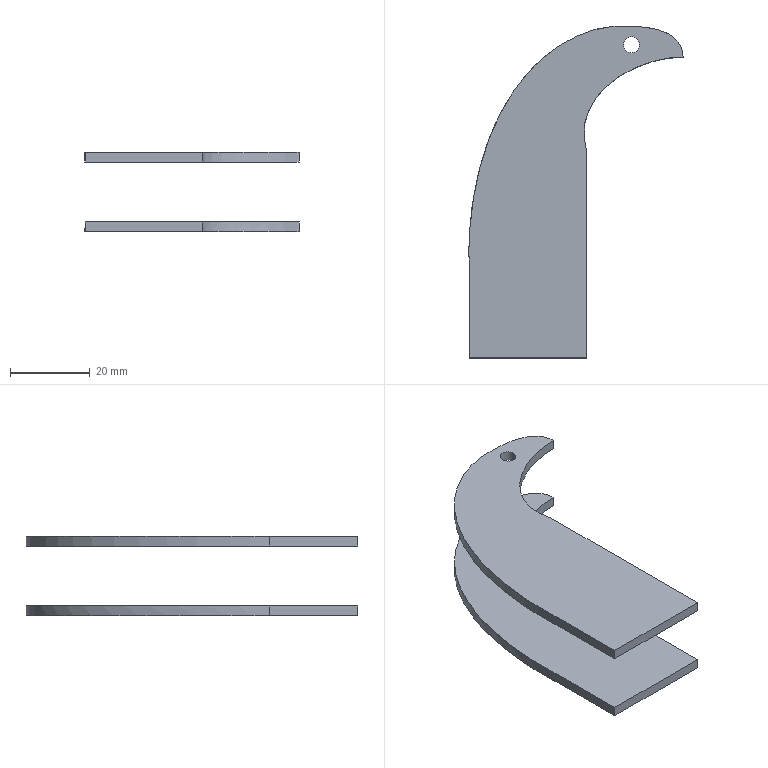Part | SolidWorks | features ICE 2, Extrusion 1 | 2 solids | 18 faces | box 53.74 x 83.25 x 20 mm | volume 11198 mm3 | plane 10 | cylinder 4 | spline 4 | commonest cylinder face diameters 4 x4
STEP:
#1=CARTESIAN_POINT('',(20.268,78.539,-10.));
#2=VERTEX_POINT('',#1);
#3=CARTESIAN_POINT('',(24.268,78.539,-10.));
#4=VERTEX_POINT('',#3);
#5=CARTESIAN_POINT('',(22.268,78.539,-10.));
#6=DIRECTION('',(0.,0.,1.));
#7=DIRECTION('',(1.,0.,0.));
#8=AXIS2_PLACEMENT_3D('',#5,#6,#7);
#9=CIRCLE('',#8,2.);
#10=EDGE_CURVE('',#2,#4,#9,.T.);
#11=ORIENTED_EDGE('',*,*,#10,.F.);
#12=CARTESIAN_POINT('',(20.268,78.539,-7.5));
#13=VERTEX_POINT('',#12);
#14=CARTESIAN_POINT('',(20.268,78.539,-90.));
#15=DIRECTION('',(0.,0.,1.));
#16=VECTOR('',#15,1000.);
#17=LINE('',#14,#16);
#18=EDGE_CURVE('',#2,#13,#17,.T.);
#19=ORIENTED_EDGE('',*,*,#18,.T.);
#20=CARTESIAN_POINT('',(24.268,78.539,-7.5));
#21=VERTEX_POINT('',#20);
#22=CARTESIAN_POINT('',(22.268,78.539,-7.5));
#23=DIRECTION('',(0.,0.,-1.));
#24=DIRECTION('',(-1.,0.,0.));
#25=AXIS2_PLACEMENT_3D('',#22,#23,#24);
#26=CIRCLE('',#25,2.);
#27=EDGE_CURVE('',#21,#13,#26,.T.);
#28=ORIENTED_EDGE('',*,*,#27,.F.);
#29=CARTESIAN_POINT('',(24.268,78.539,-90.));
#30=DIRECTION('',(0.,0.,1.));
#31=VECTOR('',#30,1000.);
#32=LINE('',#29,#31);
#33=EDGE_CURVE('',#4,#21,#32,.T.);
#34=ORIENTED_EDGE('',*,*,#33,.F.);
#35=EDGE_LOOP('',(#11,#19,#28,#34));
#36=FACE_OUTER_BOUND('',#35,.T.);
#37=CARTESIAN_POINT('',(22.268,78.539,-90.));
#38=DIRECTION('',(0.,0.,1.));
#39=DIRECTION('',(1.,0.,0.));
#40=AXIS2_PLACEMENT_3D('',#37,#38,#39);
#41=CYLINDRICAL_SURFACE('',#40,2.);
#42=ADVANCED_FACE('',(#36),#41,.F.);
#43=CARTESIAN_POINT('',(-18.438,0.,-7.5));
#44=VERTEX_POINT('',#43);
#45=CARTESIAN_POINT('',(-18.438,0.,-10.));
#46=VERTEX_POINT('',#45);
#47=CARTESIAN_POINT('',(-18.438,0.,10.));
#48=DIRECTION('',(0.,0.,-1.));
#49=VECTOR('',#48,1000.);
#50=LINE('',#47,#49);
#51=EDGE_CURVE('',#44,#46,#50,.T.);
#52=ORIENTED_EDGE('',*,*,#51,.F.);
#53=CARTESIAN_POINT('',(-18.438,22.25,-7.5));
#54=VERTEX_POINT('',#53);
#55=CARTESIAN_POINT('',(-18.438,0.,-7.5));
#56=DIRECTION('',(0.,1.,0.));
#57=VECTOR('',#56,1000.);
#58=LINE('',#55,#57);
#59=EDGE_CURVE('',#44,#54,#58,.T.);
#60=ORIENTED_EDGE('',*,*,#59,.T.);
#61=CARTESIAN_POINT('',(-18.438,22.25,-10.));
#62=VERTEX_POINT('',#61);
#63=CARTESIAN_POINT('',(-18.438,22.25,10.));
#64=DIRECTION('',(0.,0.,-1.));
#65=VECTOR('',#64,1000.);
#66=LINE('',#63,#65);
#67=EDGE_CURVE('',#54,#62,#66,.T.);
#68=ORIENTED_EDGE('',*,*,#67,.T.);
#69=CARTESIAN_POINT('',(-18.438,0.,-10.));
#70=DIRECTION('',(0.,-1.,0.));
#71=VECTOR('',#70,1000.);
#72=LINE('',#69,#71);
#73=EDGE_CURVE('',#62,#46,#72,.T.);
#74=ORIENTED_EDGE('',*,*,#73,.T.);
#75=EDGE_LOOP('',(#52,#60,#68,#74));
#76=FACE_OUTER_BOUND('',#75,.T.);
#77=CARTESIAN_POINT('',(-18.438,0.,10.));
#78=DIRECTION('',(1.,0.,0.));
#79=DIRECTION('',(0.,0.,-1.));
#80=AXIS2_PLACEMENT_3D('',#77,#78,#79);
#81=PLANE('',#80);
#82=ADVANCED_FACE('',(#76),#81,.F.);
#83=CARTESIAN_POINT('',(10.984,0.,-7.5));
#84=VERTEX_POINT('',#83);
#85=CARTESIAN_POINT('',(10.984,0.,-10.));
#86=VERTEX_POINT('',#85);
#87=CARTESIAN_POINT('',(10.984,0.,10.));
#88=DIRECTION('',(0.,0.,-1.));
#89=VECTOR('',#88,1000.);
#90=LINE('',#87,#89);
#91=EDGE_CURVE('',#84,#86,#90,.T.);
#92=ORIENTED_EDGE('',*,*,#91,.F.);
#93=CARTESIAN_POINT('',(-18.438,0.,-7.5));
#94=DIRECTION('',(-1.,0.,0.));
#95=VECTOR('',#94,1000.);
#96=LINE('',#93,#95);
#97=EDGE_CURVE('',#84,#44,#96,.T.);
#98=ORIENTED_EDGE('',*,*,#97,.T.);
#99=ORIENTED_EDGE('',*,*,#51,.T.);
#100=CARTESIAN_POINT('',(-18.438,0.,-10.));
#101=DIRECTION('',(1.,0.,0.));
#102=VECTOR('',#101,1000.);
#103=LINE('',#100,#102);
#104=EDGE_CURVE('',#46,#86,#103,.T.);
#105=ORIENTED_EDGE('',*,*,#104,.T.);
#106=EDGE_LOOP('',(#92,#98,#99,#105));
#107=FACE_OUTER_BOUND('',#106,.T.);
#108=CARTESIAN_POINT('',(-18.438,0.,10.));
#109=DIRECTION('',(0.,1.,0.));
#110=DIRECTION('',(0.,0.,1.));
#111=AXIS2_PLACEMENT_3D('',#108,#109,#110);
#112=PLANE('',#111);
#113=ADVANCED_FACE('',(#107),#112,.F.);
#114=CARTESIAN_POINT('',(10.984,52.083,-7.5));
#115=VERTEX_POINT('',#114);
#116=CARTESIAN_POINT('',(10.984,52.083,-10.));
#117=VERTEX_POINT('',#116);
#118=CARTESIAN_POINT('',(10.984,52.083,10.));
#119=DIRECTION('',(0.,0.,-1.));
#120=VECTOR('',#119,1000.);
#121=LINE('',#118,#120);
#122=EDGE_CURVE('',#115,#117,#121,.T.);
#123=ORIENTED_EDGE('',*,*,#122,.F.);
#124=CARTESIAN_POINT('',(10.984,52.083,-7.5));
#125=DIRECTION('',(0.,-1.,0.));
#126=VECTOR('',#125,1000.);
#127=LINE('',#124,#126);
#128=EDGE_CURVE('',#115,#84,#127,.T.);
#129=ORIENTED_EDGE('',*,*,#128,.T.);
#130=ORIENTED_EDGE('',*,*,#91,.T.);
#131=CARTESIAN_POINT('',(10.984,52.083,-10.));
#132=DIRECTION('',(0.,1.,0.));
#133=VECTOR('',#132,1000.);
#134=LINE('',#131,#133);
#135=EDGE_CURVE('',#86,#117,#134,.T.);
#136=ORIENTED_EDGE('',*,*,#135,.T.);
#137=EDGE_LOOP('',(#123,#129,#130,#136));
#138=FACE_OUTER_BOUND('',#137,.T.);
#139=CARTESIAN_POINT('',(10.984,52.083,10.));
#140=DIRECTION('',(-1.,0.,0.));
#141=DIRECTION('',(0.,-1.,0.));
#142=AXIS2_PLACEMENT_3D('',#139,#140,#141);
#143=PLANE('',#142);
#144=ADVANCED_FACE('',(#138),#143,.F.);
#145=CARTESIAN_POINT('',(35.215,75.441,-7.5));
#146=VERTEX_POINT('',#145);
#147=CARTESIAN_POINT('',(35.215,75.441,-10.));
#148=VERTEX_POINT('',#147);
#149=CARTESIAN_POINT('',(35.215,75.441,10.));
#150=DIRECTION('',(0.,0.,-1.));
#151=VECTOR('',#150,1000.);
#152=LINE('',#149,#151);
#153=EDGE_CURVE('',#146,#148,#152,.T.);
#154=ORIENTED_EDGE('',*,*,#153,.F.);
#155=CARTESIAN_POINT('',(35.215,75.441,-7.5));
#156=CARTESIAN_POINT('',(23.557,75.598,-7.5));
#157=CARTESIAN_POINT('',(6.934,66.328,-7.5));
#158=CARTESIAN_POINT('',(10.984,52.083,-7.5));
#159=B_SPLINE_CURVE_WITH_KNOTS('',3,(#155,#156,#157,#158),.UNSPECIFIED.,.F.,.F.,(4,4),(0.,1.),.UNSPECIFIED.);
#160=EDGE_CURVE('',#146,#115,#159,.T.);
#161=ORIENTED_EDGE('',*,*,#160,.T.);
#162=ORIENTED_EDGE('',*,*,#122,.T.);
#163=CARTESIAN_POINT('',(10.984,52.083,-10.));
#164=CARTESIAN_POINT('',(6.934,66.328,-10.));
#165=CARTESIAN_POINT('',(23.557,75.598,-10.));
#166=CARTESIAN_POINT('',(35.215,75.441,-10.));
#167=B_SPLINE_CURVE_WITH_KNOTS('',3,(#163,#164,#165,#166),.UNSPECIFIED.,.F.,.F.,(4,4),(0.,1.),.UNSPECIFIED.);
#168=EDGE_CURVE('',#117,#148,#167,.T.);
#169=ORIENTED_EDGE('',*,*,#168,.T.);
#170=EDGE_LOOP('',(#154,#161,#162,#169));
#171=FACE_OUTER_BOUND('',#170,.T.);
#172=CARTESIAN_POINT('',(10.984,52.083,-7.5));
#173=CARTESIAN_POINT('',(10.984,52.083,-10.));
#174=CARTESIAN_POINT('',(6.934,66.328,-7.5));
#175=CARTESIAN_POINT('',(6.934,66.328,-10.));
#176=CARTESIAN_POINT('',(23.557,75.598,-7.5));
#177=CARTESIAN_POINT('',(23.557,75.598,-10.));
#178=CARTESIAN_POINT('',(35.215,75.441,-7.5));
#179=CARTESIAN_POINT('',(35.215,75.441,-10.));
#180=B_SPLINE_SURFACE_WITH_KNOTS('',3,1,((#172,#173),(#174,#175),(#176,#177),(#178,#179)),.UNSPECIFIED.,.F.,.F.,.F.,(4,4),(2,2),(0.,1.),(0.,1.),.UNSPECIFIED.);
#181=ADVANCED_FACE('',(#171),#180,.F.);
#182=ORIENTED_EDGE('',*,*,#67,.F.);
#183=CARTESIAN_POINT('',(-18.438,22.25,-7.5));
#184=CARTESIAN_POINT('',(-19.279,40.919,-7.5));
#185=CARTESIAN_POINT('',(-12.619,70.796,-7.5));
#186=CARTESIAN_POINT('',(13.495,83.4,-7.5));
#187=CARTESIAN_POINT('',(23.092,83.31,-7.5));
#188=CARTESIAN_POINT('',(30.862,82.311,-7.5));
#189=CARTESIAN_POINT('',(35.305,78.999,-7.5));
#190=CARTESIAN_POINT('',(35.215,75.441,-7.5));
#191=B_SPLINE_CURVE_WITH_KNOTS('',3,(#183,#184,#185,#186,#187,#188,#189,#190),.UNSPECIFIED.,.F.,.F.,(4,1,1,1,1,4),(0.,0.6141,0.7591,0.8514,0.9042,1.),.UNSPECIFIED.);
#192=EDGE_CURVE('',#54,#146,#191,.T.);
#193=ORIENTED_EDGE('',*,*,#192,.T.);
#194=ORIENTED_EDGE('',*,*,#153,.T.);
#195=CARTESIAN_POINT('',(35.215,75.441,-10.));
#196=CARTESIAN_POINT('',(35.305,78.999,-10.));
#197=CARTESIAN_POINT('',(30.862,82.311,-10.));
#198=CARTESIAN_POINT('',(23.092,83.31,-10.));
#199=CARTESIAN_POINT('',(13.495,83.4,-10.));
#200=CARTESIAN_POINT('',(-12.619,70.796,-10.));
#201=CARTESIAN_POINT('',(-19.279,40.919,-10.));
#202=CARTESIAN_POINT('',(-18.438,22.25,-10.));
#203=B_SPLINE_CURVE_WITH_KNOTS('',3,(#195,#196,#197,#198,#199,#200,#201,#202),.UNSPECIFIED.,.F.,.F.,(4,1,1,1,1,4),(0.,0.09577,0.1486,0.2409,0.3859,1.),.UNSPECIFIED.);
#204=EDGE_CURVE('',#148,#62,#203,.T.);
#205=ORIENTED_EDGE('',*,*,#204,.T.);
#206=EDGE_LOOP('',(#182,#193,#194,#205));
#207=FACE_OUTER_BOUND('',#206,.T.);
#208=CARTESIAN_POINT('',(35.215,75.441,-7.5));
#209=CARTESIAN_POINT('',(35.215,75.441,-10.));
#210=CARTESIAN_POINT('',(35.305,78.999,-7.5));
#211=CARTESIAN_POINT('',(35.305,78.999,-10.));
#212=CARTESIAN_POINT('',(30.862,82.311,-7.5));
#213=CARTESIAN_POINT('',(30.862,82.311,-10.));
#214=CARTESIAN_POINT('',(23.092,83.31,-7.5));
#215=CARTESIAN_POINT('',(23.092,83.31,-10.));
#216=CARTESIAN_POINT('',(13.495,83.4,-7.5));
#217=CARTESIAN_POINT('',(13.495,83.4,-10.));
#218=CARTESIAN_POINT('',(-12.619,70.796,-7.5));
#219=CARTESIAN_POINT('',(-12.619,70.796,-10.));
#220=CARTESIAN_POINT('',(-19.279,40.919,-7.5));
#221=CARTESIAN_POINT('',(-19.279,40.919,-10.));
#222=CARTESIAN_POINT('',(-18.438,22.25,-7.5));
#223=CARTESIAN_POINT('',(-18.438,22.25,-10.));
#224=B_SPLINE_SURFACE_WITH_KNOTS('',3,1,((#208,#209),(#210,#211),(#212,#213),(#214,#215),(#216,#217),(#218,#219),(#220,#221),(#222,#223)),.UNSPECIFIED.,.F.,.F.,.F.,(4,1,1,1,1,4),(2,2),(0.,0.09577,0.1486,0.2409,0.3859,1.),(0.,1.),.UNSPECIFIED.);
#225=ADVANCED_FACE('',(#207),#224,.F.);
#226=CARTESIAN_POINT('',(22.268,78.539,-10.));
#227=DIRECTION('',(0.,0.,1.));
#228=DIRECTION('',(1.,0.,0.));
#229=AXIS2_PLACEMENT_3D('',#226,#227,#228);
#230=CIRCLE('',#229,2.);
#231=EDGE_CURVE('',#4,#2,#230,.T.);
#232=ORIENTED_EDGE('',*,*,#231,.T.);
#233=ORIENTED_EDGE('',*,*,#10,.T.);
#234=EDGE_LOOP('',(#232,#233));
#235=FACE_BOUND('',#234,.T.);
#236=ORIENTED_EDGE('',*,*,#73,.F.);
#237=ORIENTED_EDGE('',*,*,#204,.F.);
#238=ORIENTED_EDGE('',*,*,#168,.F.);
#239=ORIENTED_EDGE('',*,*,#135,.F.);
#240=ORIENTED_EDGE('',*,*,#104,.F.);
#241=EDGE_LOOP('',(#236,#237,#238,#239,#240));
#242=FACE_OUTER_BOUND('',#241,.T.);
#243=CARTESIAN_POINT('',(-5.594,69.238,-10.));
#244=DIRECTION('',(0.,0.,1.));
#245=DIRECTION('',(1.,0.,0.));
#246=AXIS2_PLACEMENT_3D('',#243,#244,#245);
#247=PLANE('',#246);
#248=ADVANCED_FACE('',(#235,#242),#247,.F.);
#249=ORIENTED_EDGE('',*,*,#27,.T.);
#250=CARTESIAN_POINT('',(22.268,78.539,-7.5));
#251=DIRECTION('',(0.,0.,-1.));
#252=DIRECTION('',(-1.,0.,0.));
#253=AXIS2_PLACEMENT_3D('',#250,#251,#252);
#254=CIRCLE('',#253,2.);
#255=EDGE_CURVE('',#13,#21,#254,.T.);
#256=ORIENTED_EDGE('',*,*,#255,.T.);
#257=EDGE_LOOP('',(#249,#256));
#258=FACE_BOUND('',#257,.T.);
#259=ORIENTED_EDGE('',*,*,#97,.F.);
#260=ORIENTED_EDGE('',*,*,#128,.F.);
#261=ORIENTED_EDGE('',*,*,#160,.F.);
#262=ORIENTED_EDGE('',*,*,#192,.F.);
#263=ORIENTED_EDGE('',*,*,#59,.F.);
#264=EDGE_LOOP('',(#259,#260,#261,#262,#263));
#265=FACE_OUTER_BOUND('',#264,.T.);
#266=CARTESIAN_POINT('',(-50.,-93.589,-7.5));
#267=DIRECTION('',(0.,0.,-1.));
#268=DIRECTION('',(-1.,0.,0.));
#269=AXIS2_PLACEMENT_3D('',#266,#267,#268);
#270=PLANE('',#269);
#271=ADVANCED_FACE('',(#258,#265),#270,.F.);
#272=ORIENTED_EDGE('',*,*,#18,.F.);
#273=ORIENTED_EDGE('',*,*,#231,.F.);
#274=ORIENTED_EDGE('',*,*,#33,.T.);
#275=ORIENTED_EDGE('',*,*,#255,.F.);
#276=EDGE_LOOP('',(#272,#273,#274,#275));
#277=FACE_OUTER_BOUND('',#276,.T.);
#278=CARTESIAN_POINT('',(22.268,78.539,-90.));
#279=DIRECTION('',(0.,0.,1.));
#280=DIRECTION('',(1.,0.,0.));
#281=AXIS2_PLACEMENT_3D('',#278,#279,#280);
#282=CYLINDRICAL_SURFACE('',#281,2.);
#283=ADVANCED_FACE('',(#277),#282,.F.);
#284=CLOSED_SHELL('',(#42,#82,#113,#144,#181,#225,#248,#271,#283));
#285=MANIFOLD_SOLID_BREP('',#284);
#286=CARTESIAN_POINT('',(20.268,78.539,7.5));
#287=VERTEX_POINT('',#286);
#288=CARTESIAN_POINT('',(24.268,78.539,7.5));
#289=VERTEX_POINT('',#288);
#290=CARTESIAN_POINT('',(22.268,78.539,7.5));
#291=DIRECTION('',(0.,0.,1.));
#292=DIRECTION('',(1.,0.,0.));
#293=AXIS2_PLACEMENT_3D('',#290,#291,#292);
#294=CIRCLE('',#293,2.);
#295=EDGE_CURVE('',#287,#289,#294,.T.);
#296=ORIENTED_EDGE('',*,*,#295,.F.);
#297=CARTESIAN_POINT('',(20.268,78.539,10.));
#298=VERTEX_POINT('',#297);
#299=CARTESIAN_POINT('',(20.268,78.539,-90.));
#300=DIRECTION('',(0.,0.,1.));
#301=VECTOR('',#300,1000.);
#302=LINE('',#299,#301);
#303=EDGE_CURVE('',#287,#298,#302,.T.);
#304=ORIENTED_EDGE('',*,*,#303,.T.);
#305=CARTESIAN_POINT('',(24.268,78.539,10.));
#306=VERTEX_POINT('',#305);
#307=CARTESIAN_POINT('',(22.268,78.539,10.));
#308=DIRECTION('',(0.,0.,1.));
#309=DIRECTION('',(1.,0.,0.));
#310=AXIS2_PLACEMENT_3D('',#307,#308,#309);
#311=CIRCLE('',#310,2.);
#312=EDGE_CURVE('',#298,#306,#311,.T.);
#313=ORIENTED_EDGE('',*,*,#312,.T.);
#314=CARTESIAN_POINT('',(24.268,78.539,-90.));
#315=DIRECTION('',(0.,0.,1.));
#316=VECTOR('',#315,1000.);
#317=LINE('',#314,#316);
#318=EDGE_CURVE('',#289,#306,#317,.T.);
#319=ORIENTED_EDGE('',*,*,#318,.F.);
#320=EDGE_LOOP('',(#296,#304,#313,#319));
#321=FACE_OUTER_BOUND('',#320,.T.);
#322=CARTESIAN_POINT('',(22.268,78.539,-90.));
#323=DIRECTION('',(0.,0.,1.));
#324=DIRECTION('',(1.,0.,0.));
#325=AXIS2_PLACEMENT_3D('',#322,#323,#324);
#326=CYLINDRICAL_SURFACE('',#325,2.);
#327=ADVANCED_FACE('',(#321),#326,.F.);
#328=CARTESIAN_POINT('',(22.268,78.539,10.));
#329=DIRECTION('',(0.,0.,1.));
#330=DIRECTION('',(1.,0.,0.));
#331=AXIS2_PLACEMENT_3D('',#328,#329,#330);
#332=CIRCLE('',#331,2.);
#333=EDGE_CURVE('',#306,#298,#332,.T.);
#334=ORIENTED_EDGE('',*,*,#333,.F.);
#335=ORIENTED_EDGE('',*,*,#312,.F.);
#336=EDGE_LOOP('',(#334,#335));
#337=FACE_BOUND('',#336,.T.);
#338=CARTESIAN_POINT('',(-18.438,22.25,10.));
#339=VERTEX_POINT('',#338);
#340=CARTESIAN_POINT('',(-18.438,0.,10.));
#341=VERTEX_POINT('',#340);
#342=CARTESIAN_POINT('',(-18.438,0.,10.));
#343=DIRECTION('',(0.,-1.,0.));
#344=VECTOR('',#343,1000.);
#345=LINE('',#342,#344);
#346=EDGE_CURVE('',#339,#341,#345,.T.);
#347=ORIENTED_EDGE('',*,*,#346,.T.);
#348=CARTESIAN_POINT('',(10.984,0.,10.));
#349=VERTEX_POINT('',#348);
#350=CARTESIAN_POINT('',(-18.438,0.,10.));
#351=DIRECTION('',(1.,0.,0.));
#352=VECTOR('',#351,1000.);
#353=LINE('',#350,#352);
#354=EDGE_CURVE('',#341,#349,#353,.T.);
#355=ORIENTED_EDGE('',*,*,#354,.T.);
#356=CARTESIAN_POINT('',(10.984,52.083,10.));
#357=VERTEX_POINT('',#356);
#358=CARTESIAN_POINT('',(10.984,52.083,10.));
#359=DIRECTION('',(0.,1.,0.));
#360=VECTOR('',#359,1000.);
#361=LINE('',#358,#360);
#362=EDGE_CURVE('',#349,#357,#361,.T.);
#363=ORIENTED_EDGE('',*,*,#362,.T.);
#364=CARTESIAN_POINT('',(35.215,75.441,10.));
#365=VERTEX_POINT('',#364);
#366=CARTESIAN_POINT('',(10.984,52.083,10.));
#367=CARTESIAN_POINT('',(6.934,66.328,10.));
#368=CARTESIAN_POINT('',(23.557,75.598,10.));
#369=CARTESIAN_POINT('',(35.215,75.441,10.));
#370=B_SPLINE_CURVE_WITH_KNOTS('',3,(#366,#367,#368,#369),.UNSPECIFIED.,.F.,.F.,(4,4),(0.,1.),.UNSPECIFIED.);
#371=EDGE_CURVE('',#357,#365,#370,.T.);
#372=ORIENTED_EDGE('',*,*,#371,.T.);
#373=CARTESIAN_POINT('',(35.215,75.441,10.));
#374=CARTESIAN_POINT('',(35.305,78.999,10.));
#375=CARTESIAN_POINT('',(30.862,82.311,10.));
#376=CARTESIAN_POINT('',(23.092,83.31,10.));
#377=CARTESIAN_POINT('',(13.495,83.4,10.));
#378=CARTESIAN_POINT('',(-12.619,70.796,10.));
#379=CARTESIAN_POINT('',(-19.279,40.919,10.));
#380=CARTESIAN_POINT('',(-18.438,22.25,10.));
#381=B_SPLINE_CURVE_WITH_KNOTS('',3,(#373,#374,#375,#376,#377,#378,#379,#380),.UNSPECIFIED.,.F.,.F.,(4,1,1,1,1,4),(0.,0.09577,0.1486,0.2409,0.3859,1.),.UNSPECIFIED.);
#382=EDGE_CURVE('',#365,#339,#381,.T.);
#383=ORIENTED_EDGE('',*,*,#382,.T.);
#384=EDGE_LOOP('',(#347,#355,#363,#372,#383));
#385=FACE_OUTER_BOUND('',#384,.T.);
#386=CARTESIAN_POINT('',(-5.594,69.238,10.));
#387=DIRECTION('',(0.,0.,1.));
#388=DIRECTION('',(1.,0.,0.));
#389=AXIS2_PLACEMENT_3D('',#386,#387,#388);
#390=PLANE('',#389);
#391=ADVANCED_FACE('',(#337,#385),#390,.T.);
#392=CARTESIAN_POINT('',(35.215,75.441,7.5));
#393=VERTEX_POINT('',#392);
#394=CARTESIAN_POINT('',(35.215,75.441,10.));
#395=DIRECTION('',(0.,0.,-1.));
#396=VECTOR('',#395,1000.);
#397=LINE('',#394,#396);
#398=EDGE_CURVE('',#365,#393,#397,.T.);
#399=ORIENTED_EDGE('',*,*,#398,.T.);
#400=CARTESIAN_POINT('',(-18.438,22.25,7.5));
#401=VERTEX_POINT('',#400);
#402=CARTESIAN_POINT('',(35.215,75.441,7.5));
#403=CARTESIAN_POINT('',(35.305,78.999,7.5));
#404=CARTESIAN_POINT('',(30.862,82.311,7.5));
#405=CARTESIAN_POINT('',(23.092,83.31,7.5));
#406=CARTESIAN_POINT('',(13.495,83.4,7.5));
#407=CARTESIAN_POINT('',(-12.619,70.796,7.5));
#408=CARTESIAN_POINT('',(-19.279,40.919,7.5));
#409=CARTESIAN_POINT('',(-18.438,22.25,7.5));
#410=B_SPLINE_CURVE_WITH_KNOTS('',3,(#402,#403,#404,#405,#406,#407,#408,#409),.UNSPECIFIED.,.F.,.F.,(4,1,1,1,1,4),(0.,0.09577,0.1486,0.2409,0.3859,1.),.UNSPECIFIED.);
#411=EDGE_CURVE('',#393,#401,#410,.T.);
#412=ORIENTED_EDGE('',*,*,#411,.T.);
#413=CARTESIAN_POINT('',(-18.438,22.25,10.));
#414=DIRECTION('',(0.,0.,-1.));
#415=VECTOR('',#414,1000.);
#416=LINE('',#413,#415);
#417=EDGE_CURVE('',#339,#401,#416,.T.);
#418=ORIENTED_EDGE('',*,*,#417,.F.);
#419=ORIENTED_EDGE('',*,*,#382,.F.);
#420=EDGE_LOOP('',(#399,#412,#418,#419));
#421=FACE_OUTER_BOUND('',#420,.T.);
#422=CARTESIAN_POINT('',(35.215,75.441,10.));
#423=CARTESIAN_POINT('',(35.215,75.441,7.5));
#424=CARTESIAN_POINT('',(35.305,78.999,10.));
#425=CARTESIAN_POINT('',(35.305,78.999,7.5));
#426=CARTESIAN_POINT('',(30.862,82.311,10.));
#427=CARTESIAN_POINT('',(30.862,82.311,7.5));
#428=CARTESIAN_POINT('',(23.092,83.31,10.));
#429=CARTESIAN_POINT('',(23.092,83.31,7.5));
#430=CARTESIAN_POINT('',(13.495,83.4,10.));
#431=CARTESIAN_POINT('',(13.495,83.4,7.5));
#432=CARTESIAN_POINT('',(-12.619,70.796,10.));
#433=CARTESIAN_POINT('',(-12.619,70.796,7.5));
#434=CARTESIAN_POINT('',(-19.279,40.919,10.));
#435=CARTESIAN_POINT('',(-19.279,40.919,7.5));
#436=CARTESIAN_POINT('',(-18.438,22.25,10.));
#437=CARTESIAN_POINT('',(-18.438,22.25,7.5));
#438=B_SPLINE_SURFACE_WITH_KNOTS('',3,1,((#422,#423),(#424,#425),(#426,#427),(#428,#429),(#430,#431),(#432,#433),(#434,#435),(#436,#437)),.UNSPECIFIED.,.F.,.F.,.F.,(4,1,1,1,1,4),(2,2),(0.,0.09577,0.1486,0.2409,0.3859,1.),(0.,1.),.UNSPECIFIED.);
#439=ADVANCED_FACE('',(#421),#438,.F.);
#440=CARTESIAN_POINT('',(10.984,52.083,7.5));
#441=VERTEX_POINT('',#440);
#442=CARTESIAN_POINT('',(10.984,52.083,10.));
#443=DIRECTION('',(0.,0.,-1.));
#444=VECTOR('',#443,1000.);
#445=LINE('',#442,#444);
#446=EDGE_CURVE('',#357,#441,#445,.T.);
#447=ORIENTED_EDGE('',*,*,#446,.T.);
#448=CARTESIAN_POINT('',(10.984,52.083,7.5));
#449=CARTESIAN_POINT('',(6.934,66.328,7.5));
#450=CARTESIAN_POINT('',(23.557,75.598,7.5));
#451=CARTESIAN_POINT('',(35.215,75.441,7.5));
#452=B_SPLINE_CURVE_WITH_KNOTS('',3,(#448,#449,#450,#451),.UNSPECIFIED.,.F.,.F.,(4,4),(0.,1.),.UNSPECIFIED.);
#453=EDGE_CURVE('',#441,#393,#452,.T.);
#454=ORIENTED_EDGE('',*,*,#453,.T.);
#455=ORIENTED_EDGE('',*,*,#398,.F.);
#456=ORIENTED_EDGE('',*,*,#371,.F.);
#457=EDGE_LOOP('',(#447,#454,#455,#456));
#458=FACE_OUTER_BOUND('',#457,.T.);
#459=CARTESIAN_POINT('',(10.984,52.083,10.));
#460=CARTESIAN_POINT('',(10.984,52.083,7.5));
#461=CARTESIAN_POINT('',(6.934,66.328,10.));
#462=CARTESIAN_POINT('',(6.934,66.328,7.5));
#463=CARTESIAN_POINT('',(23.557,75.598,10.));
#464=CARTESIAN_POINT('',(23.557,75.598,7.5));
#465=CARTESIAN_POINT('',(35.215,75.441,10.));
#466=CARTESIAN_POINT('',(35.215,75.441,7.5));
#467=B_SPLINE_SURFACE_WITH_KNOTS('',3,1,((#459,#460),(#461,#462),(#463,#464),(#465,#466)),.UNSPECIFIED.,.F.,.F.,.F.,(4,4),(2,2),(0.,1.),(0.,1.),.UNSPECIFIED.);
#468=ADVANCED_FACE('',(#458),#467,.F.);
#469=CARTESIAN_POINT('',(10.984,0.,7.5));
#470=VERTEX_POINT('',#469);
#471=CARTESIAN_POINT('',(10.984,0.,10.));
#472=DIRECTION('',(0.,0.,-1.));
#473=VECTOR('',#472,1000.);
#474=LINE('',#471,#473);
#475=EDGE_CURVE('',#349,#470,#474,.T.);
#476=ORIENTED_EDGE('',*,*,#475,.T.);
#477=CARTESIAN_POINT('',(10.984,52.083,7.5));
#478=DIRECTION('',(0.,1.,0.));
#479=VECTOR('',#478,1000.);
#480=LINE('',#477,#479);
#481=EDGE_CURVE('',#470,#441,#480,.T.);
#482=ORIENTED_EDGE('',*,*,#481,.T.);
#483=ORIENTED_EDGE('',*,*,#446,.F.);
#484=ORIENTED_EDGE('',*,*,#362,.F.);
#485=EDGE_LOOP('',(#476,#482,#483,#484));
#486=FACE_OUTER_BOUND('',#485,.T.);
#487=CARTESIAN_POINT('',(10.984,52.083,10.));
#488=DIRECTION('',(-1.,0.,0.));
#489=DIRECTION('',(0.,-1.,0.));
#490=AXIS2_PLACEMENT_3D('',#487,#488,#489);
#491=PLANE('',#490);
#492=ADVANCED_FACE('',(#486),#491,.F.);
#493=CARTESIAN_POINT('',(-18.438,0.,7.5));
#494=VERTEX_POINT('',#493);
#495=CARTESIAN_POINT('',(-18.438,0.,10.));
#496=DIRECTION('',(0.,0.,-1.));
#497=VECTOR('',#496,1000.);
#498=LINE('',#495,#497);
#499=EDGE_CURVE('',#341,#494,#498,.T.);
#500=ORIENTED_EDGE('',*,*,#499,.T.);
#501=CARTESIAN_POINT('',(-18.438,0.,7.5));
#502=DIRECTION('',(1.,0.,0.));
#503=VECTOR('',#502,1000.);
#504=LINE('',#501,#503);
#505=EDGE_CURVE('',#494,#470,#504,.T.);
#506=ORIENTED_EDGE('',*,*,#505,.T.);
#507=ORIENTED_EDGE('',*,*,#475,.F.);
#508=ORIENTED_EDGE('',*,*,#354,.F.);
#509=EDGE_LOOP('',(#500,#506,#507,#508));
#510=FACE_OUTER_BOUND('',#509,.T.);
#511=CARTESIAN_POINT('',(-18.438,0.,10.));
#512=DIRECTION('',(0.,1.,0.));
#513=DIRECTION('',(0.,0.,1.));
#514=AXIS2_PLACEMENT_3D('',#511,#512,#513);
#515=PLANE('',#514);
#516=ADVANCED_FACE('',(#510),#515,.F.);
#517=ORIENTED_EDGE('',*,*,#417,.T.);
#518=CARTESIAN_POINT('',(-18.438,0.,7.5));
#519=DIRECTION('',(0.,-1.,0.));
#520=VECTOR('',#519,1000.);
#521=LINE('',#518,#520);
#522=EDGE_CURVE('',#401,#494,#521,.T.);
#523=ORIENTED_EDGE('',*,*,#522,.T.);
#524=ORIENTED_EDGE('',*,*,#499,.F.);
#525=ORIENTED_EDGE('',*,*,#346,.F.);
#526=EDGE_LOOP('',(#517,#523,#524,#525));
#527=FACE_OUTER_BOUND('',#526,.T.);
#528=CARTESIAN_POINT('',(-18.438,0.,10.));
#529=DIRECTION('',(1.,0.,0.));
#530=DIRECTION('',(0.,0.,-1.));
#531=AXIS2_PLACEMENT_3D('',#528,#529,#530);
#532=PLANE('',#531);
#533=ADVANCED_FACE('',(#527),#532,.F.);
#534=CARTESIAN_POINT('',(22.268,78.539,7.5));
#535=DIRECTION('',(0.,0.,1.));
#536=DIRECTION('',(1.,0.,0.));
#537=AXIS2_PLACEMENT_3D('',#534,#535,#536);
#538=CIRCLE('',#537,2.);
#539=EDGE_CURVE('',#289,#287,#538,.T.);
#540=ORIENTED_EDGE('',*,*,#539,.T.);
#541=ORIENTED_EDGE('',*,*,#295,.T.);
#542=EDGE_LOOP('',(#540,#541));
#543=FACE_BOUND('',#542,.T.);
#544=ORIENTED_EDGE('',*,*,#411,.F.);
#545=ORIENTED_EDGE('',*,*,#453,.F.);
#546=ORIENTED_EDGE('',*,*,#481,.F.);
#547=ORIENTED_EDGE('',*,*,#505,.F.);
#548=ORIENTED_EDGE('',*,*,#522,.F.);
#549=EDGE_LOOP('',(#544,#545,#546,#547,#548));
#550=FACE_OUTER_BOUND('',#549,.T.);
#551=CARTESIAN_POINT('',(-50.,-93.589,7.5));
#552=DIRECTION('',(0.,0.,1.));
#553=DIRECTION('',(1.,0.,0.));
#554=AXIS2_PLACEMENT_3D('',#551,#552,#553);
#555=PLANE('',#554);
#556=ADVANCED_FACE('',(#543,#550),#555,.F.);
#557=ORIENTED_EDGE('',*,*,#303,.F.);
#558=ORIENTED_EDGE('',*,*,#539,.F.);
#559=ORIENTED_EDGE('',*,*,#318,.T.);
#560=ORIENTED_EDGE('',*,*,#333,.T.);
#561=EDGE_LOOP('',(#557,#558,#559,#560));
#562=FACE_OUTER_BOUND('',#561,.T.);
#563=CARTESIAN_POINT('',(22.268,78.539,-90.));
#564=DIRECTION('',(0.,0.,1.));
#565=DIRECTION('',(1.,0.,0.));
#566=AXIS2_PLACEMENT_3D('',#563,#564,#565);
#567=CYLINDRICAL_SURFACE('',#566,2.);
#568=ADVANCED_FACE('',(#562),#567,.F.);
#569=CLOSED_SHELL('',(#327,#391,#439,#468,#492,#516,#533,#556,#568));
#570=MANIFOLD_SOLID_BREP('',#569);
#571=CARTESIAN_POINT('',(0.,0.,0.));
#572=DIRECTION('',(0.,0.,1.));
#573=DIRECTION('',(1.,0.,0.));
#574=AXIS2_PLACEMENT_3D('',#571,#572,#573);
#575=(LENGTH_UNIT()NAMED_UNIT(*)SI_UNIT(.MILLI.,.METRE.));
#576=UNCERTAINTY_MEASURE_WITH_UNIT(LENGTH_MEASURE(0.00001),#575,'','');
#577=(NAMED_UNIT(*)PLANE_ANGLE_UNIT()SI_UNIT($,.RADIAN.));
#578=(NAMED_UNIT(*)SI_UNIT($,.STERADIAN.)SOLID_ANGLE_UNIT());
#579=(GEOMETRIC_REPRESENTATION_CONTEXT(3)GLOBAL_UNCERTAINTY_ASSIGNED_CONTEXT((#576))GLOBAL_UNIT_ASSIGNED_CONTEXT((#575,#577,#578))REPRESENTATION_CONTEXT('',''));
#580=ADVANCED_BREP_SHAPE_REPRESENTATION('',(#285,#570,#574),#579);